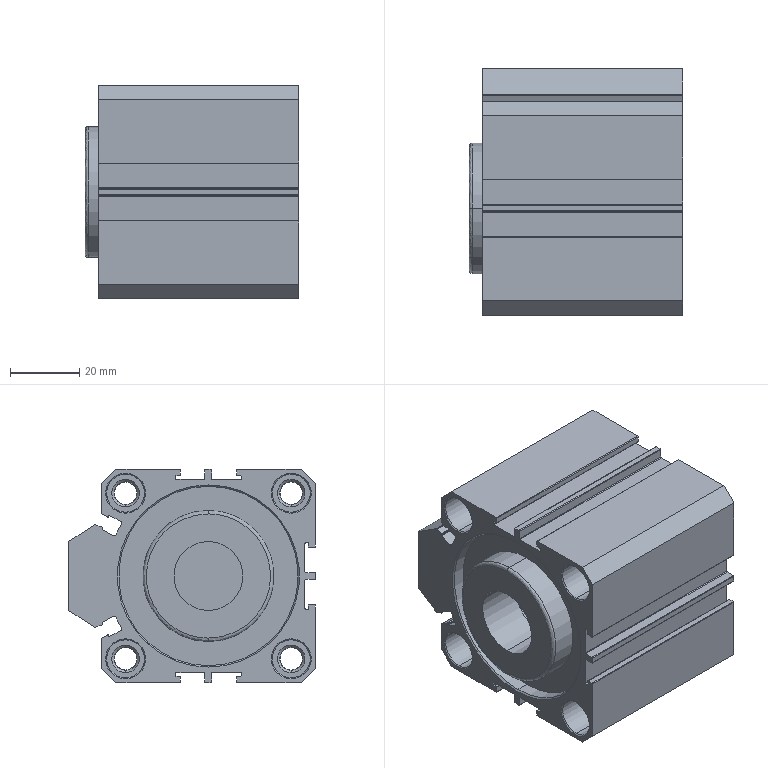Part | SolidWorks | features BaseBody 1 | 1 solid | 255 faces | box 62 x 71.5 x 62 mm | volume 122269 mm3 | cylinder 110 | plane 87 | cone 56 | spline 2 | commonest cylinder face diameters 0.4 x46 6.647 x16 11 x16 0.8 x10 6.5 x8 11.445 x4